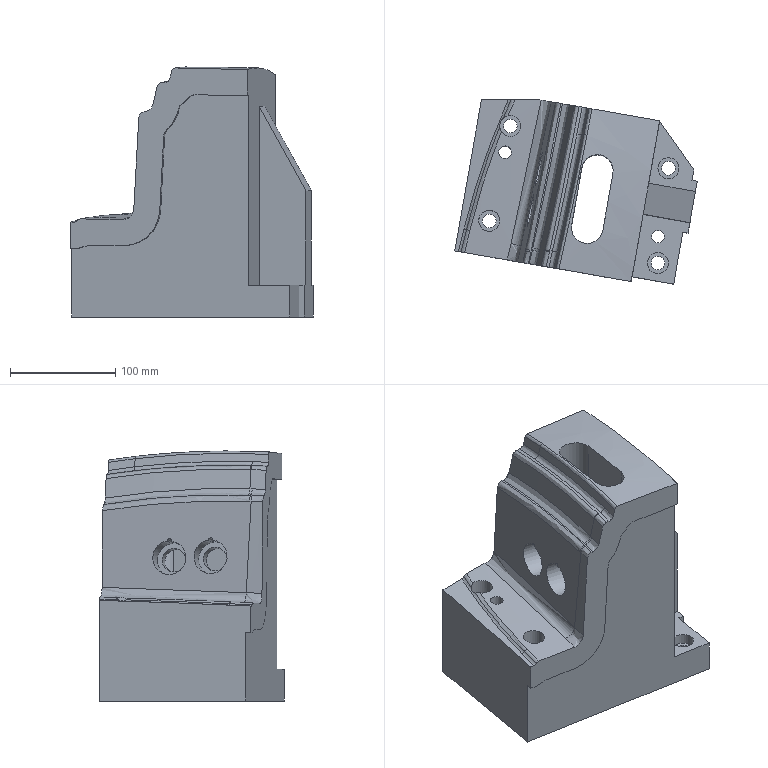Part | NX | features solid 2 | 1 solid | 80 faces | box 229.967 x 174.799 x 237.26 mm | volume 4138983 mm3 | spline 36 | plane 26 | cylinder 18 | commonest cylinder face diameters 13 x4 20 x4 4 x2 12 x2 22.6 x2 30 x2